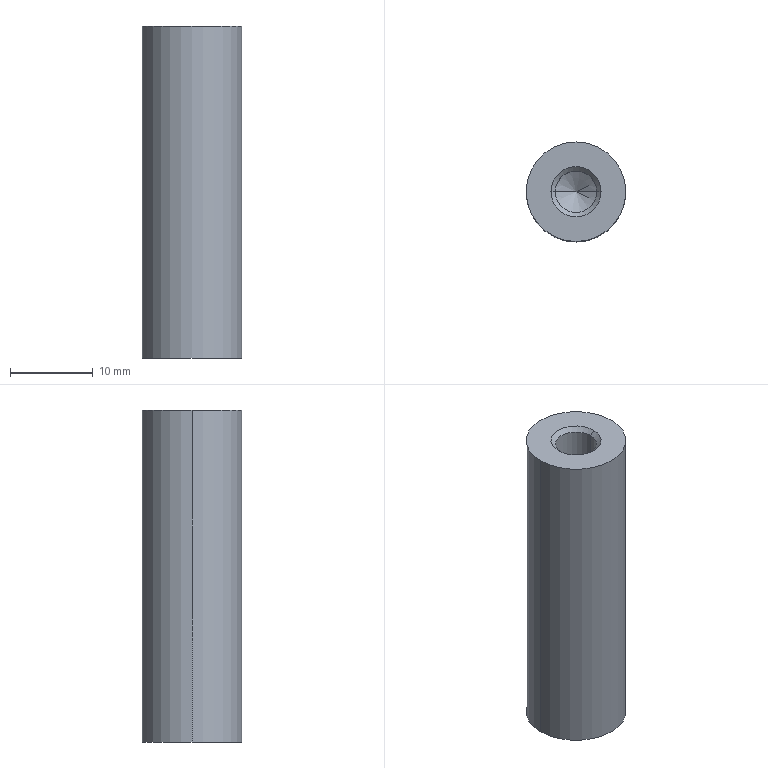Part | SolidWorks | features 3DProfileFeature 1, Extrusion 1, HoleWzd 1, MirrorPattern 1 | 1 solid | 16 faces | box 12 x 12 x 40 mm | volume 4146 mm3 | cone 8 | cylinder 6 | plane 2 | commonest cylinder face diameters 5 x4 12 x2
STEP:
#1=CARTESIAN_POINT('',(2.5,0.,-19.475));
#2=VERTEX_POINT('',#1);
#3=CARTESIAN_POINT('',(-2.5,0.,-19.475));
#4=VERTEX_POINT('',#3);
#5=CARTESIAN_POINT('',(0.,0.,-19.475));
#6=DIRECTION('',(0.,0.,-1.));
#7=DIRECTION('',(-1.,0.,0.));
#8=AXIS2_PLACEMENT_3D('',#5,#6,#7);
#9=CIRCLE('',#8,2.5);
#10=EDGE_CURVE('',#2,#4,#9,.T.);
#11=ORIENTED_EDGE('',*,*,#10,.F.);
#12=CARTESIAN_POINT('',(3.025,0.,-20.));
#13=VERTEX_POINT('',#12);
#14=CARTESIAN_POINT('',(3.025,0.,-20.));
#15=DIRECTION('',(0.7071,0.,-0.7071));
#16=VECTOR('',#15,1000.);
#17=LINE('',#14,#16);
#18=EDGE_CURVE('',#2,#13,#17,.T.);
#19=ORIENTED_EDGE('',*,*,#18,.T.);
#20=CARTESIAN_POINT('',(-3.025,0.,-20.));
#21=VERTEX_POINT('',#20);
#22=CARTESIAN_POINT('',(0.,0.,-20.));
#23=DIRECTION('',(0.,0.,-1.));
#24=DIRECTION('',(-1.,0.,0.));
#25=AXIS2_PLACEMENT_3D('',#22,#23,#24);
#26=CIRCLE('',#25,3.025);
#27=EDGE_CURVE('',#13,#21,#26,.T.);
#28=ORIENTED_EDGE('',*,*,#27,.T.);
#29=CARTESIAN_POINT('',(-3.025,0.,-20.));
#30=DIRECTION('',(-0.7071,0.,-0.7071));
#31=VECTOR('',#30,1000.);
#32=LINE('',#29,#31);
#33=EDGE_CURVE('',#4,#21,#32,.T.);
#34=ORIENTED_EDGE('',*,*,#33,.F.);
#35=EDGE_LOOP('',(#11,#19,#28,#34));
#36=FACE_OUTER_BOUND('',#35,.T.);
#37=CARTESIAN_POINT('',(0.,0.,-20.));
#38=DIRECTION('',(0.,0.,-1.));
#39=DIRECTION('',(-1.,0.,0.));
#40=AXIS2_PLACEMENT_3D('',#37,#38,#39);
#41=CONICAL_SURFACE('',#40,3.025,0.7854);
#42=ADVANCED_FACE('',(#36),#41,.F.);
#43=CARTESIAN_POINT('',(2.5,0.,-11.));
#44=VERTEX_POINT('',#43);
#45=CARTESIAN_POINT('',(-2.5,0.,-11.));
#46=VERTEX_POINT('',#45);
#47=CARTESIAN_POINT('',(0.,0.,-11.));
#48=DIRECTION('',(0.,0.,-1.));
#49=DIRECTION('',(-1.,0.,0.));
#50=AXIS2_PLACEMENT_3D('',#47,#48,#49);
#51=CIRCLE('',#50,2.5);
#52=EDGE_CURVE('',#44,#46,#51,.T.);
#53=ORIENTED_EDGE('',*,*,#52,.F.);
#54=CARTESIAN_POINT('',(2.5,0.,-20.));
#55=DIRECTION('',(0.,0.,-1.));
#56=VECTOR('',#55,1000.);
#57=LINE('',#54,#56);
#58=EDGE_CURVE('',#44,#2,#57,.T.);
#59=ORIENTED_EDGE('',*,*,#58,.T.);
#60=ORIENTED_EDGE('',*,*,#10,.T.);
#61=CARTESIAN_POINT('',(-2.5,0.,-20.));
#62=DIRECTION('',(0.,0.,-1.));
#63=VECTOR('',#62,1000.);
#64=LINE('',#61,#63);
#65=EDGE_CURVE('',#46,#4,#64,.T.);
#66=ORIENTED_EDGE('',*,*,#65,.F.);
#67=EDGE_LOOP('',(#53,#59,#60,#66));
#68=FACE_OUTER_BOUND('',#67,.T.);
#69=CARTESIAN_POINT('',(0.,0.,-20.));
#70=DIRECTION('',(0.,0.,-1.));
#71=DIRECTION('',(-1.,0.,0.));
#72=AXIS2_PLACEMENT_3D('',#69,#70,#71);
#73=CYLINDRICAL_SURFACE('',#72,2.5);
#74=ADVANCED_FACE('',(#68),#73,.F.);
#75=CARTESIAN_POINT('',(0.,0.,-9.498));
#76=VERTEX_POINT('',#75);
#77=CARTESIAN_POINT('',(-2.5,0.,-11.));
#78=DIRECTION('',(-0.8572,0.,-0.515));
#79=VECTOR('',#78,1000.);
#80=LINE('',#77,#79);
#81=EDGE_CURVE('',#76,#46,#80,.T.);
#82=ORIENTED_EDGE('',*,*,#81,.F.);
#83=CARTESIAN_POINT('',(2.5,0.,-11.));
#84=DIRECTION('',(0.8572,0.,-0.515));
#85=VECTOR('',#84,1000.);
#86=LINE('',#83,#85);
#87=EDGE_CURVE('',#76,#44,#86,.T.);
#88=ORIENTED_EDGE('',*,*,#87,.T.);
#89=ORIENTED_EDGE('',*,*,#52,.T.);
#90=EDGE_LOOP('',(#82,#88,#89));
#91=FACE_OUTER_BOUND('',#90,.T.);
#92=CARTESIAN_POINT('',(0.,0.,-11.));
#93=DIRECTION('',(0.,0.,-1.));
#94=DIRECTION('',(-1.,0.,0.));
#95=AXIS2_PLACEMENT_3D('',#92,#93,#94);
#96=CONICAL_SURFACE('',#95,2.5,1.03);
#97=ADVANCED_FACE('',(#91),#96,.F.);
#98=CARTESIAN_POINT('',(-2.5,0.,19.475));
#99=VERTEX_POINT('',#98);
#100=CARTESIAN_POINT('',(2.5,0.,19.475));
#101=VERTEX_POINT('',#100);
#102=CARTESIAN_POINT('',(0.,0.,19.475));
#103=DIRECTION('',(0.,0.,1.));
#104=DIRECTION('',(1.,0.,0.));
#105=AXIS2_PLACEMENT_3D('',#102,#103,#104);
#106=CIRCLE('',#105,2.5);
#107=EDGE_CURVE('',#99,#101,#106,.T.);
#108=ORIENTED_EDGE('',*,*,#107,.F.);
#109=CARTESIAN_POINT('',(-3.025,0.,20.));
#110=VERTEX_POINT('',#109);
#111=CARTESIAN_POINT('',(-3.025,0.,20.));
#112=DIRECTION('',(-0.7071,0.,0.7071));
#113=VECTOR('',#112,1000.);
#114=LINE('',#111,#113);
#115=EDGE_CURVE('',#99,#110,#114,.T.);
#116=ORIENTED_EDGE('',*,*,#115,.T.);
#117=CARTESIAN_POINT('',(3.025,0.,20.));
#118=VERTEX_POINT('',#117);
#119=CARTESIAN_POINT('',(0.,0.,20.));
#120=DIRECTION('',(0.,0.,1.));
#121=DIRECTION('',(1.,0.,0.));
#122=AXIS2_PLACEMENT_3D('',#119,#120,#121);
#123=CIRCLE('',#122,3.025);
#124=EDGE_CURVE('',#110,#118,#123,.T.);
#125=ORIENTED_EDGE('',*,*,#124,.T.);
#126=CARTESIAN_POINT('',(3.025,0.,20.));
#127=DIRECTION('',(0.7071,0.,0.7071));
#128=VECTOR('',#127,1000.);
#129=LINE('',#126,#128);
#130=EDGE_CURVE('',#101,#118,#129,.T.);
#131=ORIENTED_EDGE('',*,*,#130,.F.);
#132=EDGE_LOOP('',(#108,#116,#125,#131));
#133=FACE_OUTER_BOUND('',#132,.T.);
#134=CARTESIAN_POINT('',(0.,0.,20.));
#135=DIRECTION('',(0.,0.,1.));
#136=DIRECTION('',(1.,0.,0.));
#137=AXIS2_PLACEMENT_3D('',#134,#135,#136);
#138=CONICAL_SURFACE('',#137,3.025,0.7854);
#139=ADVANCED_FACE('',(#133),#138,.F.);
#140=CARTESIAN_POINT('',(-2.5,0.,11.));
#141=VERTEX_POINT('',#140);
#142=CARTESIAN_POINT('',(2.5,0.,11.));
#143=VERTEX_POINT('',#142);
#144=CARTESIAN_POINT('',(0.,0.,11.));
#145=DIRECTION('',(0.,0.,1.));
#146=DIRECTION('',(1.,0.,0.));
#147=AXIS2_PLACEMENT_3D('',#144,#145,#146);
#148=CIRCLE('',#147,2.5);
#149=EDGE_CURVE('',#141,#143,#148,.T.);
#150=ORIENTED_EDGE('',*,*,#149,.F.);
#151=CARTESIAN_POINT('',(-2.5,0.,20.));
#152=DIRECTION('',(0.,0.,1.));
#153=VECTOR('',#152,1000.);
#154=LINE('',#151,#153);
#155=EDGE_CURVE('',#141,#99,#154,.T.);
#156=ORIENTED_EDGE('',*,*,#155,.T.);
#157=ORIENTED_EDGE('',*,*,#107,.T.);
#158=CARTESIAN_POINT('',(2.5,0.,20.));
#159=DIRECTION('',(0.,0.,1.));
#160=VECTOR('',#159,1000.);
#161=LINE('',#158,#160);
#162=EDGE_CURVE('',#143,#101,#161,.T.);
#163=ORIENTED_EDGE('',*,*,#162,.F.);
#164=EDGE_LOOP('',(#150,#156,#157,#163));
#165=FACE_OUTER_BOUND('',#164,.T.);
#166=CARTESIAN_POINT('',(0.,0.,20.));
#167=DIRECTION('',(0.,0.,1.));
#168=DIRECTION('',(1.,0.,0.));
#169=AXIS2_PLACEMENT_3D('',#166,#167,#168);
#170=CYLINDRICAL_SURFACE('',#169,2.5);
#171=ADVANCED_FACE('',(#165),#170,.F.);
#172=CARTESIAN_POINT('',(0.,0.,9.498));
#173=VERTEX_POINT('',#172);
#174=CARTESIAN_POINT('',(2.5,0.,11.));
#175=DIRECTION('',(0.8572,0.,0.515));
#176=VECTOR('',#175,1000.);
#177=LINE('',#174,#176);
#178=EDGE_CURVE('',#173,#143,#177,.T.);
#179=ORIENTED_EDGE('',*,*,#178,.F.);
#180=CARTESIAN_POINT('',(-2.5,0.,11.));
#181=DIRECTION('',(-0.8572,0.,0.515));
#182=VECTOR('',#181,1000.);
#183=LINE('',#180,#182);
#184=EDGE_CURVE('',#173,#141,#183,.T.);
#185=ORIENTED_EDGE('',*,*,#184,.T.);
#186=ORIENTED_EDGE('',*,*,#149,.T.);
#187=EDGE_LOOP('',(#179,#185,#186));
#188=FACE_OUTER_BOUND('',#187,.T.);
#189=CARTESIAN_POINT('',(0.,0.,11.));
#190=DIRECTION('',(0.,0.,1.));
#191=DIRECTION('',(1.,0.,0.));
#192=AXIS2_PLACEMENT_3D('',#189,#190,#191);
#193=CONICAL_SURFACE('',#192,2.5,1.03);
#194=ADVANCED_FACE('',(#188),#193,.F.);
#195=CARTESIAN_POINT('',(6.,0.,20.));
#196=VERTEX_POINT('',#195);
#197=CARTESIAN_POINT('',(-6.,0.,20.));
#198=VERTEX_POINT('',#197);
#199=CARTESIAN_POINT('',(0.,0.,20.));
#200=DIRECTION('',(0.,0.,1.));
#201=DIRECTION('',(1.,0.,0.));
#202=AXIS2_PLACEMENT_3D('',#199,#200,#201);
#203=CIRCLE('',#202,6.);
#204=EDGE_CURVE('',#196,#198,#203,.T.);
#205=ORIENTED_EDGE('',*,*,#204,.F.);
#206=CARTESIAN_POINT('',(6.,0.,-20.));
#207=VERTEX_POINT('',#206);
#208=CARTESIAN_POINT('',(6.,0.,20.));
#209=DIRECTION('',(0.,0.,-1.));
#210=VECTOR('',#209,1000.);
#211=LINE('',#208,#210);
#212=EDGE_CURVE('',#196,#207,#211,.T.);
#213=ORIENTED_EDGE('',*,*,#212,.T.);
#214=CARTESIAN_POINT('',(-6.,0.,-20.));
#215=VERTEX_POINT('',#214);
#216=CARTESIAN_POINT('',(0.,0.,-20.));
#217=DIRECTION('',(0.,0.,1.));
#218=DIRECTION('',(1.,0.,0.));
#219=AXIS2_PLACEMENT_3D('',#216,#217,#218);
#220=CIRCLE('',#219,6.);
#221=EDGE_CURVE('',#207,#215,#220,.T.);
#222=ORIENTED_EDGE('',*,*,#221,.T.);
#223=CARTESIAN_POINT('',(-6.,0.,20.));
#224=DIRECTION('',(0.,0.,-1.));
#225=VECTOR('',#224,1000.);
#226=LINE('',#223,#225);
#227=EDGE_CURVE('',#198,#215,#226,.T.);
#228=ORIENTED_EDGE('',*,*,#227,.F.);
#229=EDGE_LOOP('',(#205,#213,#222,#228));
#230=FACE_OUTER_BOUND('',#229,.T.);
#231=CARTESIAN_POINT('',(0.,0.,20.));
#232=DIRECTION('',(0.,0.,-1.));
#233=DIRECTION('',(-1.,0.,0.));
#234=AXIS2_PLACEMENT_3D('',#231,#232,#233);
#235=CYLINDRICAL_SURFACE('',#234,6.);
#236=ADVANCED_FACE('',(#230),#235,.T.);
#237=ORIENTED_EDGE('',*,*,#212,.F.);
#238=CARTESIAN_POINT('',(0.,0.,20.));
#239=DIRECTION('',(0.,0.,1.));
#240=DIRECTION('',(1.,0.,0.));
#241=AXIS2_PLACEMENT_3D('',#238,#239,#240);
#242=CIRCLE('',#241,6.);
#243=EDGE_CURVE('',#198,#196,#242,.T.);
#244=ORIENTED_EDGE('',*,*,#243,.F.);
#245=ORIENTED_EDGE('',*,*,#227,.T.);
#246=CARTESIAN_POINT('',(0.,0.,-20.));
#247=DIRECTION('',(0.,0.,1.));
#248=DIRECTION('',(1.,0.,0.));
#249=AXIS2_PLACEMENT_3D('',#246,#247,#248);
#250=CIRCLE('',#249,6.);
#251=EDGE_CURVE('',#215,#207,#250,.T.);
#252=ORIENTED_EDGE('',*,*,#251,.T.);
#253=EDGE_LOOP('',(#237,#244,#245,#252));
#254=FACE_OUTER_BOUND('',#253,.T.);
#255=CARTESIAN_POINT('',(0.,0.,20.));
#256=DIRECTION('',(0.,0.,-1.));
#257=DIRECTION('',(-1.,0.,0.));
#258=AXIS2_PLACEMENT_3D('',#255,#256,#257);
#259=CYLINDRICAL_SURFACE('',#258,6.);
#260=ADVANCED_FACE('',(#254),#259,.T.);
#261=CARTESIAN_POINT('',(0.,0.,20.));
#262=DIRECTION('',(0.,0.,1.));
#263=DIRECTION('',(1.,0.,0.));
#264=AXIS2_PLACEMENT_3D('',#261,#262,#263);
#265=CIRCLE('',#264,3.025);
#266=EDGE_CURVE('',#118,#110,#265,.T.);
#267=ORIENTED_EDGE('',*,*,#266,.F.);
#268=ORIENTED_EDGE('',*,*,#124,.F.);
#269=EDGE_LOOP('',(#267,#268));
#270=FACE_BOUND('',#269,.T.);
#271=ORIENTED_EDGE('',*,*,#243,.T.);
#272=ORIENTED_EDGE('',*,*,#204,.T.);
#273=EDGE_LOOP('',(#271,#272));
#274=FACE_OUTER_BOUND('',#273,.T.);
#275=CARTESIAN_POINT('',(0.,0.,20.));
#276=DIRECTION('',(0.,0.,1.));
#277=DIRECTION('',(1.,0.,0.));
#278=AXIS2_PLACEMENT_3D('',#275,#276,#277);
#279=PLANE('',#278);
#280=ADVANCED_FACE('',(#270,#274),#279,.T.);
#281=CARTESIAN_POINT('',(0.,0.,-20.));
#282=DIRECTION('',(0.,0.,-1.));
#283=DIRECTION('',(-1.,0.,0.));
#284=AXIS2_PLACEMENT_3D('',#281,#282,#283);
#285=CIRCLE('',#284,3.025);
#286=EDGE_CURVE('',#21,#13,#285,.T.);
#287=ORIENTED_EDGE('',*,*,#286,.F.);
#288=ORIENTED_EDGE('',*,*,#27,.F.);
#289=EDGE_LOOP('',(#287,#288));
#290=FACE_BOUND('',#289,.T.);
#291=ORIENTED_EDGE('',*,*,#251,.F.);
#292=ORIENTED_EDGE('',*,*,#221,.F.);
#293=EDGE_LOOP('',(#291,#292));
#294=FACE_OUTER_BOUND('',#293,.T.);
#295=CARTESIAN_POINT('',(0.,0.,-20.));
#296=DIRECTION('',(0.,0.,1.));
#297=DIRECTION('',(1.,0.,0.));
#298=AXIS2_PLACEMENT_3D('',#295,#296,#297);
#299=PLANE('',#298);
#300=ADVANCED_FACE('',(#290,#294),#299,.F.);
#301=ORIENTED_EDGE('',*,*,#184,.F.);
#302=ORIENTED_EDGE('',*,*,#178,.T.);
#303=CARTESIAN_POINT('',(0.,0.,11.));
#304=DIRECTION('',(0.,0.,1.));
#305=DIRECTION('',(1.,0.,0.));
#306=AXIS2_PLACEMENT_3D('',#303,#304,#305);
#307=CIRCLE('',#306,2.5);
#308=EDGE_CURVE('',#143,#141,#307,.T.);
#309=ORIENTED_EDGE('',*,*,#308,.T.);
#310=EDGE_LOOP('',(#301,#302,#309));
#311=FACE_OUTER_BOUND('',#310,.T.);
#312=CARTESIAN_POINT('',(0.,0.,11.));
#313=DIRECTION('',(0.,0.,1.));
#314=DIRECTION('',(1.,0.,0.));
#315=AXIS2_PLACEMENT_3D('',#312,#313,#314);
#316=CONICAL_SURFACE('',#315,2.5,1.03);
#317=ADVANCED_FACE('',(#311),#316,.F.);
#318=ORIENTED_EDGE('',*,*,#155,.F.);
#319=ORIENTED_EDGE('',*,*,#308,.F.);
#320=ORIENTED_EDGE('',*,*,#162,.T.);
#321=CARTESIAN_POINT('',(0.,0.,19.475));
#322=DIRECTION('',(0.,0.,1.));
#323=DIRECTION('',(1.,0.,0.));
#324=AXIS2_PLACEMENT_3D('',#321,#322,#323);
#325=CIRCLE('',#324,2.5);
#326=EDGE_CURVE('',#101,#99,#325,.T.);
#327=ORIENTED_EDGE('',*,*,#326,.T.);
#328=EDGE_LOOP('',(#318,#319,#320,#327));
#329=FACE_OUTER_BOUND('',#328,.T.);
#330=CARTESIAN_POINT('',(0.,0.,20.));
#331=DIRECTION('',(0.,0.,1.));
#332=DIRECTION('',(1.,0.,0.));
#333=AXIS2_PLACEMENT_3D('',#330,#331,#332);
#334=CYLINDRICAL_SURFACE('',#333,2.5);
#335=ADVANCED_FACE('',(#329),#334,.F.);
#336=ORIENTED_EDGE('',*,*,#115,.F.);
#337=ORIENTED_EDGE('',*,*,#326,.F.);
#338=ORIENTED_EDGE('',*,*,#130,.T.);
#339=ORIENTED_EDGE('',*,*,#266,.T.);
#340=EDGE_LOOP('',(#336,#337,#338,#339));
#341=FACE_OUTER_BOUND('',#340,.T.);
#342=CARTESIAN_POINT('',(0.,0.,20.));
#343=DIRECTION('',(0.,0.,1.));
#344=DIRECTION('',(1.,0.,0.));
#345=AXIS2_PLACEMENT_3D('',#342,#343,#344);
#346=CONICAL_SURFACE('',#345,3.025,0.7854);
#347=ADVANCED_FACE('',(#341),#346,.F.);
#348=ORIENTED_EDGE('',*,*,#87,.F.);
#349=ORIENTED_EDGE('',*,*,#81,.T.);
#350=CARTESIAN_POINT('',(0.,0.,-11.));
#351=DIRECTION('',(0.,0.,-1.));
#352=DIRECTION('',(-1.,0.,0.));
#353=AXIS2_PLACEMENT_3D('',#350,#351,#352);
#354=CIRCLE('',#353,2.5);
#355=EDGE_CURVE('',#46,#44,#354,.T.);
#356=ORIENTED_EDGE('',*,*,#355,.T.);
#357=EDGE_LOOP('',(#348,#349,#356));
#358=FACE_OUTER_BOUND('',#357,.T.);
#359=CARTESIAN_POINT('',(0.,0.,-11.));
#360=DIRECTION('',(0.,0.,-1.));
#361=DIRECTION('',(-1.,0.,0.));
#362=AXIS2_PLACEMENT_3D('',#359,#360,#361);
#363=CONICAL_SURFACE('',#362,2.5,1.03);
#364=ADVANCED_FACE('',(#358),#363,.F.);
#365=ORIENTED_EDGE('',*,*,#58,.F.);
#366=ORIENTED_EDGE('',*,*,#355,.F.);
#367=ORIENTED_EDGE('',*,*,#65,.T.);
#368=CARTESIAN_POINT('',(0.,0.,-19.475));
#369=DIRECTION('',(0.,0.,-1.));
#370=DIRECTION('',(-1.,0.,0.));
#371=AXIS2_PLACEMENT_3D('',#368,#369,#370);
#372=CIRCLE('',#371,2.5);
#373=EDGE_CURVE('',#4,#2,#372,.T.);
#374=ORIENTED_EDGE('',*,*,#373,.T.);
#375=EDGE_LOOP('',(#365,#366,#367,#374));
#376=FACE_OUTER_BOUND('',#375,.T.);
#377=CARTESIAN_POINT('',(0.,0.,-20.));
#378=DIRECTION('',(0.,0.,-1.));
#379=DIRECTION('',(-1.,0.,0.));
#380=AXIS2_PLACEMENT_3D('',#377,#378,#379);
#381=CYLINDRICAL_SURFACE('',#380,2.5);
#382=ADVANCED_FACE('',(#376),#381,.F.);
#383=ORIENTED_EDGE('',*,*,#18,.F.);
#384=ORIENTED_EDGE('',*,*,#373,.F.);
#385=ORIENTED_EDGE('',*,*,#33,.T.);
#386=ORIENTED_EDGE('',*,*,#286,.T.);
#387=EDGE_LOOP('',(#383,#384,#385,#386));
#388=FACE_OUTER_BOUND('',#387,.T.);
#389=CARTESIAN_POINT('',(0.,0.,-20.));
#390=DIRECTION('',(0.,0.,-1.));
#391=DIRECTION('',(-1.,0.,0.));
#392=AXIS2_PLACEMENT_3D('',#389,#390,#391);
#393=CONICAL_SURFACE('',#392,3.025,0.7854);
#394=ADVANCED_FACE('',(#388),#393,.F.);
#395=CLOSED_SHELL('',(#42,#74,#97,#139,#171,#194,#236,#260,#280,#300,#317,#335,#347,#364,#382,#394));
#396=MANIFOLD_SOLID_BREP('',#395);
#397=CARTESIAN_POINT('',(0.,0.,0.));
#398=DIRECTION('',(0.,0.,1.));
#399=DIRECTION('',(1.,0.,0.));
#400=AXIS2_PLACEMENT_3D('',#397,#398,#399);
#401=(LENGTH_UNIT()NAMED_UNIT(*)SI_UNIT(.MILLI.,.METRE.));
#402=UNCERTAINTY_MEASURE_WITH_UNIT(LENGTH_MEASURE(0.00001),#401,'','');
#403=(NAMED_UNIT(*)PLANE_ANGLE_UNIT()SI_UNIT($,.RADIAN.));
#404=(NAMED_UNIT(*)SI_UNIT($,.STERADIAN.)SOLID_ANGLE_UNIT());
#405=(GEOMETRIC_REPRESENTATION_CONTEXT(3)GLOBAL_UNCERTAINTY_ASSIGNED_CONTEXT((#402))GLOBAL_UNIT_ASSIGNED_CONTEXT((#401,#403,#404))REPRESENTATION_CONTEXT('',''));
#406=ADVANCED_BREP_SHAPE_REPRESENTATION('',(#396,#400),#405);